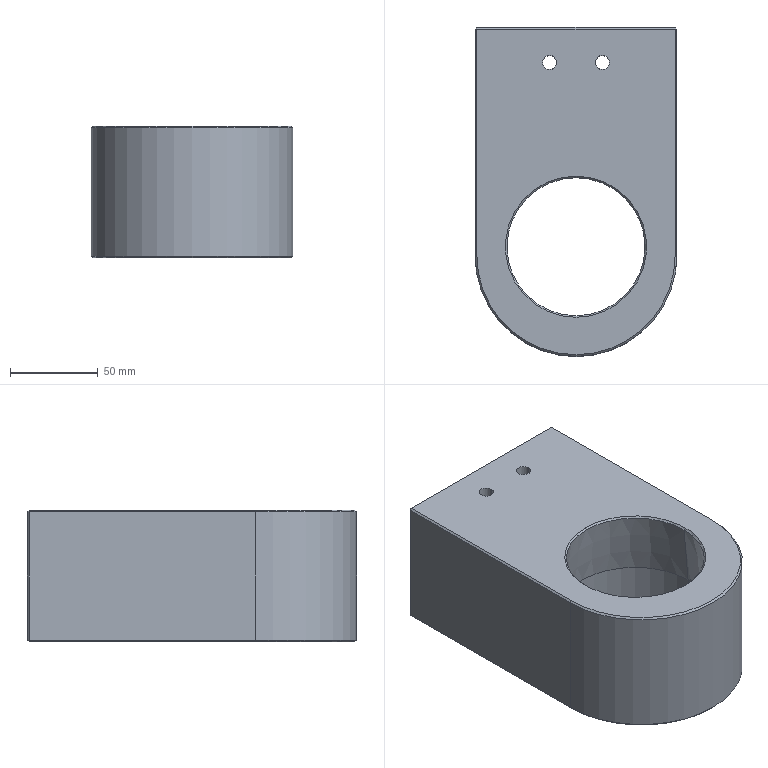Part | SolidWorks | features BaseBody 1 | 1 solid | 48 faces | box 115 x 187.5 x 75 mm | volume 1043413 mm3 | plane 24 | cone 13 | cylinder 11 | commonest cylinder face diameters 8 x4 85 x4 30 x2 115 x1